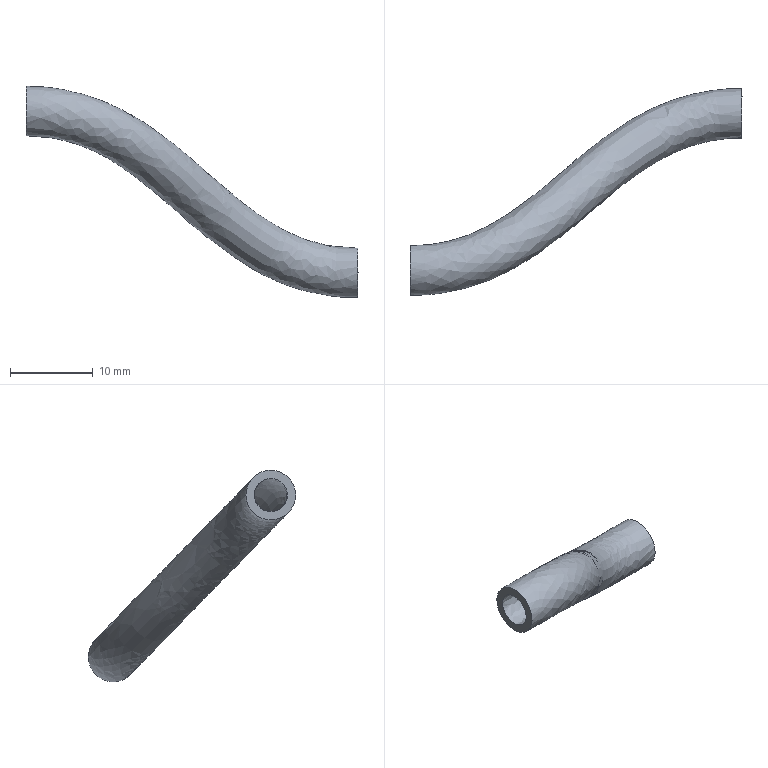Part | NX | features solid 2 | 1 solid | 4 faces | box 40.02 x 25 x 25.5 mm | volume 788.463 mm3 | plane 2 | spline 2